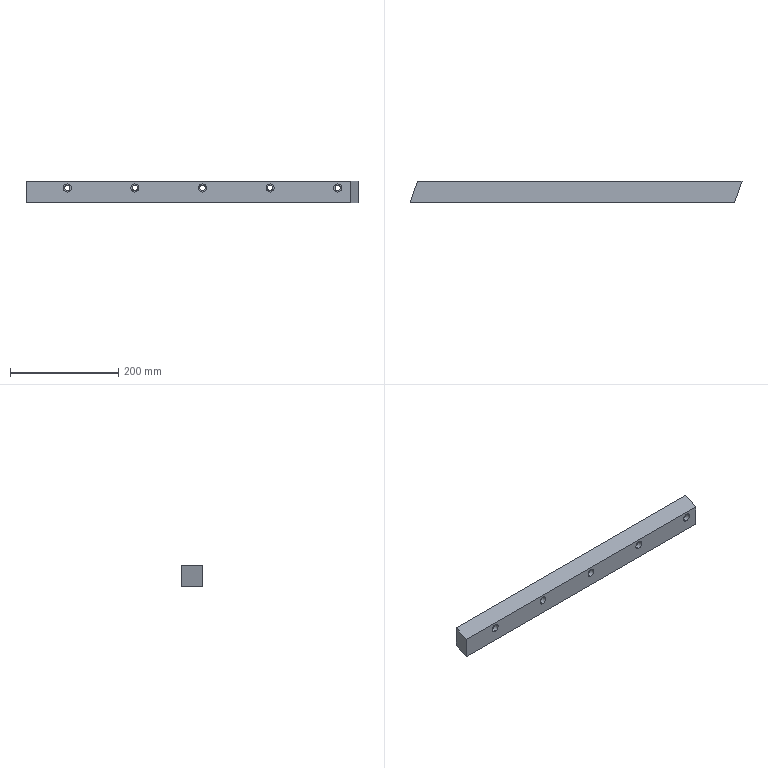Part | STEP file | MHH043906 | 1 solid | 31 faces | box 613.8 x 39 x 39 mm | volume 892867 mm3 | cylinder 20 | plane 11 | commonest cylinder face diameters 10 x10 15 x10
STEP:
#1=CARTESIAN_POINT('',(187.5,-30.,34.5));
#2=VERTEX_POINT('',#1);
#3=CARTESIAN_POINT('',(187.5,-30.,19.5));
#4=VERTEX_POINT('',#3);
#5=CARTESIAN_POINT('',(187.5,-30.,27.));
#6=DIRECTION('',(0.,-1.,0.));
#7=DIRECTION('',(0.,0.,-1.));
#8=AXIS2_PLACEMENT_3D('',#5,#6,#7);
#9=CIRCLE('',#8,7.5);
#10=EDGE_CURVE('',#2,#4,#9,.T.);
#11=ORIENTED_EDGE('',*,*,#10,.F.);
#12=CARTESIAN_POINT('',(187.5,-39.,34.5));
#13=VERTEX_POINT('',#12);
#14=CARTESIAN_POINT('',(187.5,-39.,34.5));
#15=DIRECTION('',(0.,-1.,0.));
#16=VECTOR('',#15,1000.);
#17=LINE('',#14,#16);
#18=EDGE_CURVE('',#2,#13,#17,.T.);
#19=ORIENTED_EDGE('',*,*,#18,.T.);
#20=CARTESIAN_POINT('',(187.5,-39.,19.5));
#21=VERTEX_POINT('',#20);
#22=CARTESIAN_POINT('',(187.5,-39.,27.));
#23=DIRECTION('',(0.,-1.,0.));
#24=DIRECTION('',(0.,0.,-1.));
#25=AXIS2_PLACEMENT_3D('',#22,#23,#24);
#26=CIRCLE('',#25,7.5);
#27=EDGE_CURVE('',#13,#21,#26,.T.);
#28=ORIENTED_EDGE('',*,*,#27,.T.);
#29=CARTESIAN_POINT('',(187.5,-39.,19.5));
#30=DIRECTION('',(0.,-1.,0.));
#31=VECTOR('',#30,1000.);
#32=LINE('',#29,#31);
#33=EDGE_CURVE('',#4,#21,#32,.T.);
#34=ORIENTED_EDGE('',*,*,#33,.F.);
#35=EDGE_LOOP('',(#11,#19,#28,#34));
#36=FACE_OUTER_BOUND('',#35,.T.);
#37=CARTESIAN_POINT('',(187.5,-39.,27.));
#38=DIRECTION('',(0.,-1.,0.));
#39=DIRECTION('',(0.,0.,-1.));
#40=AXIS2_PLACEMENT_3D('',#37,#38,#39);
#41=CYLINDRICAL_SURFACE('',#40,7.5);
#42=ADVANCED_FACE('',(#36),#41,.F.);
#43=CARTESIAN_POINT('',(187.5,0.,32.));
#44=VERTEX_POINT('',#43);
#45=CARTESIAN_POINT('',(187.5,0.,22.));
#46=VERTEX_POINT('',#45);
#47=CARTESIAN_POINT('',(187.5,0.,27.));
#48=DIRECTION('',(0.,-1.,0.));
#49=DIRECTION('',(0.,0.,-1.));
#50=AXIS2_PLACEMENT_3D('',#47,#48,#49);
#51=CIRCLE('',#50,5.);
#52=EDGE_CURVE('',#44,#46,#51,.T.);
#53=ORIENTED_EDGE('',*,*,#52,.F.);
#54=CARTESIAN_POINT('',(187.5,-30.,32.));
#55=VERTEX_POINT('',#54);
#56=CARTESIAN_POINT('',(187.5,-39.,32.));
#57=DIRECTION('',(0.,-1.,0.));
#58=VECTOR('',#57,1000.);
#59=LINE('',#56,#58);
#60=EDGE_CURVE('',#44,#55,#59,.T.);
#61=ORIENTED_EDGE('',*,*,#60,.T.);
#62=CARTESIAN_POINT('',(187.5,-30.,22.));
#63=VERTEX_POINT('',#62);
#64=CARTESIAN_POINT('',(187.5,-30.,27.));
#65=DIRECTION('',(0.,-1.,0.));
#66=DIRECTION('',(0.,0.,-1.));
#67=AXIS2_PLACEMENT_3D('',#64,#65,#66);
#68=CIRCLE('',#67,5.);
#69=EDGE_CURVE('',#55,#63,#68,.T.);
#70=ORIENTED_EDGE('',*,*,#69,.T.);
#71=CARTESIAN_POINT('',(187.5,-39.,22.));
#72=DIRECTION('',(0.,-1.,0.));
#73=VECTOR('',#72,1000.);
#74=LINE('',#71,#73);
#75=EDGE_CURVE('',#46,#63,#74,.T.);
#76=ORIENTED_EDGE('',*,*,#75,.F.);
#77=EDGE_LOOP('',(#53,#61,#70,#76));
#78=FACE_OUTER_BOUND('',#77,.T.);
#79=CARTESIAN_POINT('',(187.5,-39.,27.));
#80=DIRECTION('',(0.,-1.,0.));
#81=DIRECTION('',(0.,0.,-1.));
#82=AXIS2_PLACEMENT_3D('',#79,#80,#81);
#83=CYLINDRICAL_SURFACE('',#82,5.);
#84=ADVANCED_FACE('',(#78),#83,.F.);
#85=CARTESIAN_POINT('',(62.5,-30.,34.5));
#86=VERTEX_POINT('',#85);
#87=CARTESIAN_POINT('',(62.5,-30.,19.5));
#88=VERTEX_POINT('',#87);
#89=CARTESIAN_POINT('',(62.5,-30.,27.));
#90=DIRECTION('',(0.,-1.,0.));
#91=DIRECTION('',(0.,0.,-1.));
#92=AXIS2_PLACEMENT_3D('',#89,#90,#91);
#93=CIRCLE('',#92,7.5);
#94=EDGE_CURVE('',#86,#88,#93,.T.);
#95=ORIENTED_EDGE('',*,*,#94,.F.);
#96=CARTESIAN_POINT('',(62.5,-39.,34.5));
#97=VERTEX_POINT('',#96);
#98=CARTESIAN_POINT('',(62.5,-39.,34.5));
#99=DIRECTION('',(0.,-1.,0.));
#100=VECTOR('',#99,1000.);
#101=LINE('',#98,#100);
#102=EDGE_CURVE('',#86,#97,#101,.T.);
#103=ORIENTED_EDGE('',*,*,#102,.T.);
#104=CARTESIAN_POINT('',(62.5,-39.,19.5));
#105=VERTEX_POINT('',#104);
#106=CARTESIAN_POINT('',(62.5,-39.,27.));
#107=DIRECTION('',(0.,-1.,0.));
#108=DIRECTION('',(0.,0.,-1.));
#109=AXIS2_PLACEMENT_3D('',#106,#107,#108);
#110=CIRCLE('',#109,7.5);
#111=EDGE_CURVE('',#97,#105,#110,.T.);
#112=ORIENTED_EDGE('',*,*,#111,.T.);
#113=CARTESIAN_POINT('',(62.5,-39.,19.5));
#114=DIRECTION('',(0.,-1.,0.));
#115=VECTOR('',#114,1000.);
#116=LINE('',#113,#115);
#117=EDGE_CURVE('',#88,#105,#116,.T.);
#118=ORIENTED_EDGE('',*,*,#117,.F.);
#119=EDGE_LOOP('',(#95,#103,#112,#118));
#120=FACE_OUTER_BOUND('',#119,.T.);
#121=CARTESIAN_POINT('',(62.5,-39.,27.));
#122=DIRECTION('',(0.,-1.,0.));
#123=DIRECTION('',(0.,0.,-1.));
#124=AXIS2_PLACEMENT_3D('',#121,#122,#123);
#125=CYLINDRICAL_SURFACE('',#124,7.5);
#126=ADVANCED_FACE('',(#120),#125,.F.);
#127=CARTESIAN_POINT('',(62.5,0.,32.));
#128=VERTEX_POINT('',#127);
#129=CARTESIAN_POINT('',(62.5,0.,22.));
#130=VERTEX_POINT('',#129);
#131=CARTESIAN_POINT('',(62.5,0.,27.));
#132=DIRECTION('',(0.,-1.,0.));
#133=DIRECTION('',(0.,0.,-1.));
#134=AXIS2_PLACEMENT_3D('',#131,#132,#133);
#135=CIRCLE('',#134,5.);
#136=EDGE_CURVE('',#128,#130,#135,.T.);
#137=ORIENTED_EDGE('',*,*,#136,.F.);
#138=CARTESIAN_POINT('',(62.5,-30.,32.));
#139=VERTEX_POINT('',#138);
#140=CARTESIAN_POINT('',(62.5,-39.,32.));
#141=DIRECTION('',(0.,-1.,0.));
#142=VECTOR('',#141,1000.);
#143=LINE('',#140,#142);
#144=EDGE_CURVE('',#128,#139,#143,.T.);
#145=ORIENTED_EDGE('',*,*,#144,.T.);
#146=CARTESIAN_POINT('',(62.5,-30.,22.));
#147=VERTEX_POINT('',#146);
#148=CARTESIAN_POINT('',(62.5,-30.,27.));
#149=DIRECTION('',(0.,-1.,0.));
#150=DIRECTION('',(0.,0.,-1.));
#151=AXIS2_PLACEMENT_3D('',#148,#149,#150);
#152=CIRCLE('',#151,5.);
#153=EDGE_CURVE('',#139,#147,#152,.T.);
#154=ORIENTED_EDGE('',*,*,#153,.T.);
#155=CARTESIAN_POINT('',(62.5,-39.,22.));
#156=DIRECTION('',(0.,-1.,0.));
#157=VECTOR('',#156,1000.);
#158=LINE('',#155,#157);
#159=EDGE_CURVE('',#130,#147,#158,.T.);
#160=ORIENTED_EDGE('',*,*,#159,.F.);
#161=EDGE_LOOP('',(#137,#145,#154,#160));
#162=FACE_OUTER_BOUND('',#161,.T.);
#163=CARTESIAN_POINT('',(62.5,-39.,27.));
#164=DIRECTION('',(0.,-1.,0.));
#165=DIRECTION('',(0.,0.,-1.));
#166=AXIS2_PLACEMENT_3D('',#163,#164,#165);
#167=CYLINDRICAL_SURFACE('',#166,5.);
#168=ADVANCED_FACE('',(#162),#167,.F.);
#169=CARTESIAN_POINT('',(312.5,0.,32.));
#170=VERTEX_POINT('',#169);
#171=CARTESIAN_POINT('',(312.5,0.,22.));
#172=VERTEX_POINT('',#171);
#173=CARTESIAN_POINT('',(312.5,0.,27.));
#174=DIRECTION('',(0.,-1.,0.));
#175=DIRECTION('',(0.,0.,-1.));
#176=AXIS2_PLACEMENT_3D('',#173,#174,#175);
#177=CIRCLE('',#176,5.);
#178=EDGE_CURVE('',#170,#172,#177,.T.);
#179=ORIENTED_EDGE('',*,*,#178,.F.);
#180=CARTESIAN_POINT('',(312.5,-30.,32.));
#181=VERTEX_POINT('',#180);
#182=CARTESIAN_POINT('',(312.5,-39.,32.));
#183=DIRECTION('',(0.,-1.,0.));
#184=VECTOR('',#183,1000.);
#185=LINE('',#182,#184);
#186=EDGE_CURVE('',#170,#181,#185,.T.);
#187=ORIENTED_EDGE('',*,*,#186,.T.);
#188=CARTESIAN_POINT('',(312.5,-30.,22.));
#189=VERTEX_POINT('',#188);
#190=CARTESIAN_POINT('',(312.5,-30.,27.));
#191=DIRECTION('',(0.,-1.,0.));
#192=DIRECTION('',(0.,0.,-1.));
#193=AXIS2_PLACEMENT_3D('',#190,#191,#192);
#194=CIRCLE('',#193,5.);
#195=EDGE_CURVE('',#181,#189,#194,.T.);
#196=ORIENTED_EDGE('',*,*,#195,.T.);
#197=CARTESIAN_POINT('',(312.5,-39.,22.));
#198=DIRECTION('',(0.,-1.,0.));
#199=VECTOR('',#198,1000.);
#200=LINE('',#197,#199);
#201=EDGE_CURVE('',#172,#189,#200,.T.);
#202=ORIENTED_EDGE('',*,*,#201,.F.);
#203=EDGE_LOOP('',(#179,#187,#196,#202));
#204=FACE_OUTER_BOUND('',#203,.T.);
#205=CARTESIAN_POINT('',(312.5,-39.,27.));
#206=DIRECTION('',(0.,-1.,0.));
#207=DIRECTION('',(0.,0.,-1.));
#208=AXIS2_PLACEMENT_3D('',#205,#206,#207);
#209=CYLINDRICAL_SURFACE('',#208,5.);
#210=ADVANCED_FACE('',(#204),#209,.F.);
#211=CARTESIAN_POINT('',(312.5,-30.,34.5));
#212=VERTEX_POINT('',#211);
#213=CARTESIAN_POINT('',(312.5,-30.,19.5));
#214=VERTEX_POINT('',#213);
#215=CARTESIAN_POINT('',(312.5,-30.,27.));
#216=DIRECTION('',(0.,-1.,0.));
#217=DIRECTION('',(0.,0.,-1.));
#218=AXIS2_PLACEMENT_3D('',#215,#216,#217);
#219=CIRCLE('',#218,7.5);
#220=EDGE_CURVE('',#212,#214,#219,.T.);
#221=ORIENTED_EDGE('',*,*,#220,.F.);
#222=CARTESIAN_POINT('',(312.5,-39.,34.5));
#223=VERTEX_POINT('',#222);
#224=CARTESIAN_POINT('',(312.5,-39.,34.5));
#225=DIRECTION('',(0.,-1.,0.));
#226=VECTOR('',#225,1000.);
#227=LINE('',#224,#226);
#228=EDGE_CURVE('',#212,#223,#227,.T.);
#229=ORIENTED_EDGE('',*,*,#228,.T.);
#230=CARTESIAN_POINT('',(312.5,-39.,19.5));
#231=VERTEX_POINT('',#230);
#232=CARTESIAN_POINT('',(312.5,-39.,27.));
#233=DIRECTION('',(0.,-1.,0.));
#234=DIRECTION('',(0.,0.,-1.));
#235=AXIS2_PLACEMENT_3D('',#232,#233,#234);
#236=CIRCLE('',#235,7.5);
#237=EDGE_CURVE('',#223,#231,#236,.T.);
#238=ORIENTED_EDGE('',*,*,#237,.T.);
#239=CARTESIAN_POINT('',(312.5,-39.,19.5));
#240=DIRECTION('',(0.,-1.,0.));
#241=VECTOR('',#240,1000.);
#242=LINE('',#239,#241);
#243=EDGE_CURVE('',#214,#231,#242,.T.);
#244=ORIENTED_EDGE('',*,*,#243,.F.);
#245=EDGE_LOOP('',(#221,#229,#238,#244));
#246=FACE_OUTER_BOUND('',#245,.T.);
#247=CARTESIAN_POINT('',(312.5,-39.,27.));
#248=DIRECTION('',(0.,-1.,0.));
#249=DIRECTION('',(0.,0.,-1.));
#250=AXIS2_PLACEMENT_3D('',#247,#248,#249);
#251=CYLINDRICAL_SURFACE('',#250,7.5);
#252=ADVANCED_FACE('',(#246),#251,.F.);
#253=CARTESIAN_POINT('',(437.5,0.,32.));
#254=VERTEX_POINT('',#253);
#255=CARTESIAN_POINT('',(437.5,0.,22.));
#256=VERTEX_POINT('',#255);
#257=CARTESIAN_POINT('',(437.5,0.,27.));
#258=DIRECTION('',(0.,-1.,0.));
#259=DIRECTION('',(0.,0.,-1.));
#260=AXIS2_PLACEMENT_3D('',#257,#258,#259);
#261=CIRCLE('',#260,5.);
#262=EDGE_CURVE('',#254,#256,#261,.T.);
#263=ORIENTED_EDGE('',*,*,#262,.F.);
#264=CARTESIAN_POINT('',(437.5,-30.,32.));
#265=VERTEX_POINT('',#264);
#266=CARTESIAN_POINT('',(437.5,-39.,32.));
#267=DIRECTION('',(0.,-1.,0.));
#268=VECTOR('',#267,1000.);
#269=LINE('',#266,#268);
#270=EDGE_CURVE('',#254,#265,#269,.T.);
#271=ORIENTED_EDGE('',*,*,#270,.T.);
#272=CARTESIAN_POINT('',(437.5,-30.,22.));
#273=VERTEX_POINT('',#272);
#274=CARTESIAN_POINT('',(437.5,-30.,27.));
#275=DIRECTION('',(0.,-1.,0.));
#276=DIRECTION('',(0.,0.,-1.));
#277=AXIS2_PLACEMENT_3D('',#274,#275,#276);
#278=CIRCLE('',#277,5.);
#279=EDGE_CURVE('',#265,#273,#278,.T.);
#280=ORIENTED_EDGE('',*,*,#279,.T.);
#281=CARTESIAN_POINT('',(437.5,-39.,22.));
#282=DIRECTION('',(0.,-1.,0.));
#283=VECTOR('',#282,1000.);
#284=LINE('',#281,#283);
#285=EDGE_CURVE('',#256,#273,#284,.T.);
#286=ORIENTED_EDGE('',*,*,#285,.F.);
#287=EDGE_LOOP('',(#263,#271,#280,#286));
#288=FACE_OUTER_BOUND('',#287,.T.);
#289=CARTESIAN_POINT('',(437.5,-39.,27.));
#290=DIRECTION('',(0.,-1.,0.));
#291=DIRECTION('',(0.,0.,-1.));
#292=AXIS2_PLACEMENT_3D('',#289,#290,#291);
#293=CYLINDRICAL_SURFACE('',#292,5.);
#294=ADVANCED_FACE('',(#288),#293,.F.);
#295=CARTESIAN_POINT('',(437.5,-30.,34.5));
#296=VERTEX_POINT('',#295);
#297=CARTESIAN_POINT('',(437.5,-30.,19.5));
#298=VERTEX_POINT('',#297);
#299=CARTESIAN_POINT('',(437.5,-30.,27.));
#300=DIRECTION('',(0.,-1.,0.));
#301=DIRECTION('',(0.,0.,-1.));
#302=AXIS2_PLACEMENT_3D('',#299,#300,#301);
#303=CIRCLE('',#302,7.5);
#304=EDGE_CURVE('',#296,#298,#303,.T.);
#305=ORIENTED_EDGE('',*,*,#304,.F.);
#306=CARTESIAN_POINT('',(437.5,-39.,34.5));
#307=VERTEX_POINT('',#306);
#308=CARTESIAN_POINT('',(437.5,-39.,34.5));
#309=DIRECTION('',(0.,-1.,0.));
#310=VECTOR('',#309,1000.);
#311=LINE('',#308,#310);
#312=EDGE_CURVE('',#296,#307,#311,.T.);
#313=ORIENTED_EDGE('',*,*,#312,.T.);
#314=CARTESIAN_POINT('',(437.5,-39.,19.5));
#315=VERTEX_POINT('',#314);
#316=CARTESIAN_POINT('',(437.5,-39.,27.));
#317=DIRECTION('',(0.,-1.,0.));
#318=DIRECTION('',(0.,0.,-1.));
#319=AXIS2_PLACEMENT_3D('',#316,#317,#318);
#320=CIRCLE('',#319,7.5);
#321=EDGE_CURVE('',#307,#315,#320,.T.);
#322=ORIENTED_EDGE('',*,*,#321,.T.);
#323=CARTESIAN_POINT('',(437.5,-39.,19.5));
#324=DIRECTION('',(0.,-1.,0.));
#325=VECTOR('',#324,1000.);
#326=LINE('',#323,#325);
#327=EDGE_CURVE('',#298,#315,#326,.T.);
#328=ORIENTED_EDGE('',*,*,#327,.F.);
#329=EDGE_LOOP('',(#305,#313,#322,#328));
#330=FACE_OUTER_BOUND('',#329,.T.);
#331=CARTESIAN_POINT('',(437.5,-39.,27.));
#332=DIRECTION('',(0.,-1.,0.));
#333=DIRECTION('',(0.,0.,-1.));
#334=AXIS2_PLACEMENT_3D('',#331,#332,#333);
#335=CYLINDRICAL_SURFACE('',#334,7.5);
#336=ADVANCED_FACE('',(#330),#335,.F.);
#337=CARTESIAN_POINT('',(562.5,0.,32.));
#338=VERTEX_POINT('',#337);
#339=CARTESIAN_POINT('',(562.5,0.,22.));
#340=VERTEX_POINT('',#339);
#341=CARTESIAN_POINT('',(562.5,0.,27.));
#342=DIRECTION('',(0.,-1.,0.));
#343=DIRECTION('',(0.,0.,-1.));
#344=AXIS2_PLACEMENT_3D('',#341,#342,#343);
#345=CIRCLE('',#344,5.);
#346=EDGE_CURVE('',#338,#340,#345,.T.);
#347=ORIENTED_EDGE('',*,*,#346,.F.);
#348=CARTESIAN_POINT('',(562.5,-30.,32.));
#349=VERTEX_POINT('',#348);
#350=CARTESIAN_POINT('',(562.5,-39.,32.));
#351=DIRECTION('',(0.,-1.,0.));
#352=VECTOR('',#351,1000.);
#353=LINE('',#350,#352);
#354=EDGE_CURVE('',#338,#349,#353,.T.);
#355=ORIENTED_EDGE('',*,*,#354,.T.);
#356=CARTESIAN_POINT('',(562.5,-30.,22.));
#357=VERTEX_POINT('',#356);
#358=CARTESIAN_POINT('',(562.5,-30.,27.));
#359=DIRECTION('',(0.,-1.,0.));
#360=DIRECTION('',(0.,0.,-1.));
#361=AXIS2_PLACEMENT_3D('',#358,#359,#360);
#362=CIRCLE('',#361,5.);
#363=EDGE_CURVE('',#349,#357,#362,.T.);
#364=ORIENTED_EDGE('',*,*,#363,.T.);
#365=CARTESIAN_POINT('',(562.5,-39.,22.));
#366=DIRECTION('',(0.,-1.,0.));
#367=VECTOR('',#366,1000.);
#368=LINE('',#365,#367);
#369=EDGE_CURVE('',#340,#357,#368,.T.);
#370=ORIENTED_EDGE('',*,*,#369,.F.);
#371=EDGE_LOOP('',(#347,#355,#364,#370));
#372=FACE_OUTER_BOUND('',#371,.T.);
#373=CARTESIAN_POINT('',(562.5,-39.,27.));
#374=DIRECTION('',(0.,-1.,0.));
#375=DIRECTION('',(0.,0.,-1.));
#376=AXIS2_PLACEMENT_3D('',#373,#374,#375);
#377=CYLINDRICAL_SURFACE('',#376,5.);
#378=ADVANCED_FACE('',(#372),#377,.F.);
#379=CARTESIAN_POINT('',(562.5,-30.,34.5));
#380=VERTEX_POINT('',#379);
#381=CARTESIAN_POINT('',(562.5,-30.,19.5));
#382=VERTEX_POINT('',#381);
#383=CARTESIAN_POINT('',(562.5,-30.,27.));
#384=DIRECTION('',(0.,-1.,0.));
#385=DIRECTION('',(0.,0.,-1.));
#386=AXIS2_PLACEMENT_3D('',#383,#384,#385);
#387=CIRCLE('',#386,7.5);
#388=EDGE_CURVE('',#380,#382,#387,.T.);
#389=ORIENTED_EDGE('',*,*,#388,.F.);
#390=CARTESIAN_POINT('',(562.5,-39.,34.5));
#391=VERTEX_POINT('',#390);
#392=CARTESIAN_POINT('',(562.5,-39.,34.5));
#393=DIRECTION('',(0.,-1.,0.));
#394=VECTOR('',#393,1000.);
#395=LINE('',#392,#394);
#396=EDGE_CURVE('',#380,#391,#395,.T.);
#397=ORIENTED_EDGE('',*,*,#396,.T.);
#398=CARTESIAN_POINT('',(562.5,-39.,19.5));
#399=VERTEX_POINT('',#398);
#400=CARTESIAN_POINT('',(562.5,-39.,27.));
#401=DIRECTION('',(0.,-1.,0.));
#402=DIRECTION('',(0.,0.,-1.));
#403=AXIS2_PLACEMENT_3D('',#400,#401,#402);
#404=CIRCLE('',#403,7.5);
#405=EDGE_CURVE('',#391,#399,#404,.T.);
#406=ORIENTED_EDGE('',*,*,#405,.T.);
#407=CARTESIAN_POINT('',(562.5,-39.,19.5));
#408=DIRECTION('',(0.,-1.,0.));
#409=VECTOR('',#408,1000.);
#410=LINE('',#407,#409);
#411=EDGE_CURVE('',#382,#399,#410,.T.);
#412=ORIENTED_EDGE('',*,*,#411,.F.);
#413=EDGE_LOOP('',(#389,#397,#406,#412));
#414=FACE_OUTER_BOUND('',#413,.T.);
#415=CARTESIAN_POINT('',(562.5,-39.,27.));
#416=DIRECTION('',(0.,-1.,0.));
#417=DIRECTION('',(0.,0.,-1.));
#418=AXIS2_PLACEMENT_3D('',#415,#416,#417);
#419=CYLINDRICAL_SURFACE('',#418,7.5);
#420=ADVANCED_FACE('',(#414),#419,.F.);
#421=ORIENTED_EDGE('',*,*,#396,.F.);
#422=CARTESIAN_POINT('',(562.5,-30.,27.));
#423=DIRECTION('',(0.,-1.,0.));
#424=DIRECTION('',(0.,0.,-1.));
#425=AXIS2_PLACEMENT_3D('',#422,#423,#424);
#426=CIRCLE('',#425,7.5);
#427=EDGE_CURVE('',#382,#380,#426,.T.);
#428=ORIENTED_EDGE('',*,*,#427,.F.);
#429=ORIENTED_EDGE('',*,*,#411,.T.);
#430=CARTESIAN_POINT('',(562.5,-39.,27.));
#431=DIRECTION('',(0.,-1.,0.));
#432=DIRECTION('',(0.,0.,-1.));
#433=AXIS2_PLACEMENT_3D('',#430,#431,#432);
#434=CIRCLE('',#433,7.5);
#435=EDGE_CURVE('',#399,#391,#434,.T.);
#436=ORIENTED_EDGE('',*,*,#435,.T.);
#437=EDGE_LOOP('',(#421,#428,#429,#436));
#438=FACE_OUTER_BOUND('',#437,.T.);
#439=CARTESIAN_POINT('',(562.5,-39.,27.));
#440=DIRECTION('',(0.,-1.,0.));
#441=DIRECTION('',(0.,0.,-1.));
#442=AXIS2_PLACEMENT_3D('',#439,#440,#441);
#443=CYLINDRICAL_SURFACE('',#442,7.5);
#444=ADVANCED_FACE('',(#438),#443,.F.);
#445=CARTESIAN_POINT('',(562.5,-30.,27.));
#446=DIRECTION('',(0.,-1.,0.));
#447=DIRECTION('',(0.,0.,-1.));
#448=AXIS2_PLACEMENT_3D('',#445,#446,#447);
#449=CIRCLE('',#448,5.);
#450=EDGE_CURVE('',#357,#349,#449,.T.);
#451=ORIENTED_EDGE('',*,*,#450,.F.);
#452=ORIENTED_EDGE('',*,*,#363,.F.);
#453=EDGE_LOOP('',(#451,#452));
#454=FACE_BOUND('',#453,.T.);
#455=ORIENTED_EDGE('',*,*,#427,.T.);
#456=ORIENTED_EDGE('',*,*,#388,.T.);
#457=EDGE_LOOP('',(#455,#456));
#458=FACE_OUTER_BOUND('',#457,.T.);
#459=CARTESIAN_POINT('',(567.5,-30.,27.));
#460=DIRECTION('',(0.,1.,0.));
#461=DIRECTION('',(0.,0.,1.));
#462=AXIS2_PLACEMENT_3D('',#459,#460,#461);
#463=PLANE('',#462);
#464=ADVANCED_FACE('',(#454,#458),#463,.F.);
#465=ORIENTED_EDGE('',*,*,#354,.F.);
#466=CARTESIAN_POINT('',(562.5,0.,27.));
#467=DIRECTION('',(0.,-1.,0.));
#468=DIRECTION('',(0.,0.,-1.));
#469=AXIS2_PLACEMENT_3D('',#466,#467,#468);
#470=CIRCLE('',#469,5.);
#471=EDGE_CURVE('',#340,#338,#470,.T.);
#472=ORIENTED_EDGE('',*,*,#471,.F.);
#473=ORIENTED_EDGE('',*,*,#369,.T.);
#474=ORIENTED_EDGE('',*,*,#450,.T.);
#475=EDGE_LOOP('',(#465,#472,#473,#474));
#476=FACE_OUTER_BOUND('',#475,.T.);
#477=CARTESIAN_POINT('',(562.5,-39.,27.));
#478=DIRECTION('',(0.,-1.,0.));
#479=DIRECTION('',(0.,0.,-1.));
#480=AXIS2_PLACEMENT_3D('',#477,#478,#479);
#481=CYLINDRICAL_SURFACE('',#480,5.);
#482=ADVANCED_FACE('',(#476),#481,.F.);
#483=ORIENTED_EDGE('',*,*,#312,.F.);
#484=CARTESIAN_POINT('',(437.5,-30.,27.));
#485=DIRECTION('',(0.,-1.,0.));
#486=DIRECTION('',(0.,0.,-1.));
#487=AXIS2_PLACEMENT_3D('',#484,#485,#486);
#488=CIRCLE('',#487,7.5);
#489=EDGE_CURVE('',#298,#296,#488,.T.);
#490=ORIENTED_EDGE('',*,*,#489,.F.);
#491=ORIENTED_EDGE('',*,*,#327,.T.);
#492=CARTESIAN_POINT('',(437.5,-39.,27.));
#493=DIRECTION('',(0.,-1.,0.));
#494=DIRECTION('',(0.,0.,-1.));
#495=AXIS2_PLACEMENT_3D('',#492,#493,#494);
#496=CIRCLE('',#495,7.5);
#497=EDGE_CURVE('',#315,#307,#496,.T.);
#498=ORIENTED_EDGE('',*,*,#497,.T.);
#499=EDGE_LOOP('',(#483,#490,#491,#498));
#500=FACE_OUTER_BOUND('',#499,.T.);
#501=CARTESIAN_POINT('',(437.5,-39.,27.));
#502=DIRECTION('',(0.,-1.,0.));
#503=DIRECTION('',(0.,0.,-1.));
#504=AXIS2_PLACEMENT_3D('',#501,#502,#503);
#505=CYLINDRICAL_SURFACE('',#504,7.5);
#506=ADVANCED_FACE('',(#500),#505,.F.);
#507=CARTESIAN_POINT('',(437.5,-30.,27.));
#508=DIRECTION('',(0.,-1.,0.));
#509=DIRECTION('',(0.,0.,-1.));
#510=AXIS2_PLACEMENT_3D('',#507,#508,#509);
#511=CIRCLE('',#510,5.);
#512=EDGE_CURVE('',#273,#265,#511,.T.);
#513=ORIENTED_EDGE('',*,*,#512,.F.);
#514=ORIENTED_EDGE('',*,*,#279,.F.);
#515=EDGE_LOOP('',(#513,#514));
#516=FACE_BOUND('',#515,.T.);
#517=ORIENTED_EDGE('',*,*,#489,.T.);
#518=ORIENTED_EDGE('',*,*,#304,.T.);
#519=EDGE_LOOP('',(#517,#518));
#520=FACE_OUTER_BOUND('',#519,.T.);
#521=CARTESIAN_POINT('',(442.5,-30.,27.));
#522=DIRECTION('',(0.,1.,0.));
#523=DIRECTION('',(0.,0.,1.));
#524=AXIS2_PLACEMENT_3D('',#521,#522,#523);
#525=PLANE('',#524);
#526=ADVANCED_FACE('',(#516,#520),#525,.F.);
#527=ORIENTED_EDGE('',*,*,#270,.F.);
#528=CARTESIAN_POINT('',(437.5,0.,27.));
#529=DIRECTION('',(0.,-1.,0.));
#530=DIRECTION('',(0.,0.,-1.));
#531=AXIS2_PLACEMENT_3D('',#528,#529,#530);
#532=CIRCLE('',#531,5.);
#533=EDGE_CURVE('',#256,#254,#532,.T.);
#534=ORIENTED_EDGE('',*,*,#533,.F.);
#535=ORIENTED_EDGE('',*,*,#285,.T.);
#536=ORIENTED_EDGE('',*,*,#512,.T.);
#537=EDGE_LOOP('',(#527,#534,#535,#536));
#538=FACE_OUTER_BOUND('',#537,.T.);
#539=CARTESIAN_POINT('',(437.5,-39.,27.));
#540=DIRECTION('',(0.,-1.,0.));
#541=DIRECTION('',(0.,0.,-1.));
#542=AXIS2_PLACEMENT_3D('',#539,#540,#541);
#543=CYLINDRICAL_SURFACE('',#542,5.);
#544=ADVANCED_FACE('',(#538),#543,.F.);
#545=ORIENTED_EDGE('',*,*,#228,.F.);
#546=CARTESIAN_POINT('',(312.5,-30.,27.));
#547=DIRECTION('',(0.,-1.,0.));
#548=DIRECTION('',(0.,0.,-1.));
#549=AXIS2_PLACEMENT_3D('',#546,#547,#548);
#550=CIRCLE('',#549,7.5);
#551=EDGE_CURVE('',#214,#212,#550,.T.);
#552=ORIENTED_EDGE('',*,*,#551,.F.);
#553=ORIENTED_EDGE('',*,*,#243,.T.);
#554=CARTESIAN_POINT('',(312.5,-39.,27.));
#555=DIRECTION('',(0.,-1.,0.));
#556=DIRECTION('',(0.,0.,-1.));
#557=AXIS2_PLACEMENT_3D('',#554,#555,#556);
#558=CIRCLE('',#557,7.5);
#559=EDGE_CURVE('',#231,#223,#558,.T.);
#560=ORIENTED_EDGE('',*,*,#559,.T.);
#561=EDGE_LOOP('',(#545,#552,#553,#560));
#562=FACE_OUTER_BOUND('',#561,.T.);
#563=CARTESIAN_POINT('',(312.5,-39.,27.));
#564=DIRECTION('',(0.,-1.,0.));
#565=DIRECTION('',(0.,0.,-1.));
#566=AXIS2_PLACEMENT_3D('',#563,#564,#565);
#567=CYLINDRICAL_SURFACE('',#566,7.5);
#568=ADVANCED_FACE('',(#562),#567,.F.);
#569=CARTESIAN_POINT('',(312.5,-30.,27.));
#570=DIRECTION('',(0.,-1.,0.));
#571=DIRECTION('',(0.,0.,-1.));
#572=AXIS2_PLACEMENT_3D('',#569,#570,#571);
#573=CIRCLE('',#572,5.);
#574=EDGE_CURVE('',#189,#181,#573,.T.);
#575=ORIENTED_EDGE('',*,*,#574,.F.);
#576=ORIENTED_EDGE('',*,*,#195,.F.);
#577=EDGE_LOOP('',(#575,#576));
#578=FACE_BOUND('',#577,.T.);
#579=ORIENTED_EDGE('',*,*,#551,.T.);
#580=ORIENTED_EDGE('',*,*,#220,.T.);
#581=EDGE_LOOP('',(#579,#580));
#582=FACE_OUTER_BOUND('',#581,.T.);
#583=CARTESIAN_POINT('',(317.5,-30.,27.));
#584=DIRECTION('',(0.,1.,0.));
#585=DIRECTION('',(0.,0.,1.));
#586=AXIS2_PLACEMENT_3D('',#583,#584,#585);
#587=PLANE('',#586);
#588=ADVANCED_FACE('',(#578,#582),#587,.F.);
#589=ORIENTED_EDGE('',*,*,#186,.F.);
#590=CARTESIAN_POINT('',(312.5,0.,27.));
#591=DIRECTION('',(0.,-1.,0.));
#592=DIRECTION('',(0.,0.,-1.));
#593=AXIS2_PLACEMENT_3D('',#590,#591,#592);
#594=CIRCLE('',#593,5.);
#595=EDGE_CURVE('',#172,#170,#594,.T.);
#596=ORIENTED_EDGE('',*,*,#595,.F.);
#597=ORIENTED_EDGE('',*,*,#201,.T.);
#598=ORIENTED_EDGE('',*,*,#574,.T.);
#599=EDGE_LOOP('',(#589,#596,#597,#598));
#600=FACE_OUTER_BOUND('',#599,.T.);
#601=CARTESIAN_POINT('',(312.5,-39.,27.));
#602=DIRECTION('',(0.,-1.,0.));
#603=DIRECTION('',(0.,0.,-1.));
#604=AXIS2_PLACEMENT_3D('',#601,#602,#603);
#605=CYLINDRICAL_SURFACE('',#604,5.);
#606=ADVANCED_FACE('',(#600),#605,.F.);
#607=CARTESIAN_POINT('',(187.5,0.,27.));
#608=DIRECTION('',(0.,-1.,0.));
#609=DIRECTION('',(0.,0.,-1.));
#610=AXIS2_PLACEMENT_3D('',#607,#608,#609);
#611=CIRCLE('',#610,5.);
#612=EDGE_CURVE('',#46,#44,#611,.T.);
#613=ORIENTED_EDGE('',*,*,#612,.T.);
#614=ORIENTED_EDGE('',*,*,#52,.T.);
#615=EDGE_LOOP('',(#613,#614));
#616=FACE_BOUND('',#615,.T.);
#617=CARTESIAN_POINT('',(62.5,0.,27.));
#618=DIRECTION('',(0.,-1.,0.));
#619=DIRECTION('',(0.,0.,-1.));
#620=AXIS2_PLACEMENT_3D('',#617,#618,#619);
#621=CIRCLE('',#620,5.);
#622=EDGE_CURVE('',#130,#128,#621,.T.);
#623=ORIENTED_EDGE('',*,*,#622,.T.);
#624=ORIENTED_EDGE('',*,*,#136,.T.);
#625=EDGE_LOOP('',(#623,#624));
#626=FACE_BOUND('',#625,.T.);
#627=CARTESIAN_POINT('',(600.,0.,0.));
#628=VERTEX_POINT('',#627);
#629=CARTESIAN_POINT('',(0.,0.,0.));
#630=VERTEX_POINT('',#629);
#631=CARTESIAN_POINT('',(600.,0.,0.));
#632=DIRECTION('',(-1.,0.,0.));
#633=VECTOR('',#632,1000.);
#634=LINE('',#631,#633);
#635=EDGE_CURVE('',#628,#630,#634,.T.);
#636=ORIENTED_EDGE('',*,*,#635,.T.);
#637=CARTESIAN_POINT('',(0.,0.,39.));
#638=VERTEX_POINT('',#637);
#639=CARTESIAN_POINT('',(0.,0.,39.));
#640=DIRECTION('',(0.,0.,-1.));
#641=VECTOR('',#640,1000.);
#642=LINE('',#639,#641);
#643=EDGE_CURVE('',#638,#630,#642,.T.);
#644=ORIENTED_EDGE('',*,*,#643,.F.);
#645=CARTESIAN_POINT('',(600.,0.,39.));
#646=VERTEX_POINT('',#645);
#647=CARTESIAN_POINT('',(600.,0.,39.));
#648=DIRECTION('',(-1.,0.,0.));
#649=VECTOR('',#648,1000.);
#650=LINE('',#647,#649);
#651=EDGE_CURVE('',#646,#638,#650,.T.);
#652=ORIENTED_EDGE('',*,*,#651,.F.);
#653=CARTESIAN_POINT('',(600.,0.,39.));
#654=DIRECTION('',(0.,0.,-1.));
#655=VECTOR('',#654,1000.);
#656=LINE('',#653,#655);
#657=EDGE_CURVE('',#646,#628,#656,.T.);
#658=ORIENTED_EDGE('',*,*,#657,.T.);
#659=EDGE_LOOP('',(#636,#644,#652,#658));
#660=FACE_OUTER_BOUND('',#659,.T.);
#661=ORIENTED_EDGE('',*,*,#595,.T.);
#662=ORIENTED_EDGE('',*,*,#178,.T.);
#663=EDGE_LOOP('',(#661,#662));
#664=FACE_BOUND('',#663,.T.);
#665=ORIENTED_EDGE('',*,*,#533,.T.);
#666=ORIENTED_EDGE('',*,*,#262,.T.);
#667=EDGE_LOOP('',(#665,#666));
#668=FACE_BOUND('',#667,.T.);
#669=ORIENTED_EDGE('',*,*,#471,.T.);
#670=ORIENTED_EDGE('',*,*,#346,.T.);
#671=EDGE_LOOP('',(#669,#670));
#672=FACE_BOUND('',#671,.T.);
#673=CARTESIAN_POINT('',(600.,0.,39.));
#674=DIRECTION('',(0.,-1.,0.));
#675=DIRECTION('',(1.,0.,0.));
#676=AXIS2_PLACEMENT_3D('',#673,#674,#675);
#677=PLANE('',#676);
#678=ADVANCED_FACE('',(#616,#626,#660,#664,#668,#672),#677,.F.);
#679=CARTESIAN_POINT('',(-13.8,-39.,0.));
#680=VERTEX_POINT('',#679);
#681=CARTESIAN_POINT('',(0.,0.,0.));
#682=DIRECTION('',(-0.3336,-0.9427,0.));
#683=VECTOR('',#682,1000.);
#684=LINE('',#681,#683);
#685=EDGE_CURVE('',#630,#680,#684,.T.);
#686=ORIENTED_EDGE('',*,*,#685,.T.);
#687=CARTESIAN_POINT('',(-13.8,-39.,39.));
#688=VERTEX_POINT('',#687);
#689=CARTESIAN_POINT('',(-13.8,-39.,39.));
#690=DIRECTION('',(0.,0.,-1.));
#691=VECTOR('',#690,1000.);
#692=LINE('',#689,#691);
#693=EDGE_CURVE('',#688,#680,#692,.T.);
#694=ORIENTED_EDGE('',*,*,#693,.F.);
#695=CARTESIAN_POINT('',(0.,0.,39.));
#696=DIRECTION('',(-0.3336,-0.9427,0.));
#697=VECTOR('',#696,1000.);
#698=LINE('',#695,#697);
#699=EDGE_CURVE('',#638,#688,#698,.T.);
#700=ORIENTED_EDGE('',*,*,#699,.F.);
#701=ORIENTED_EDGE('',*,*,#643,.T.);
#702=EDGE_LOOP('',(#686,#694,#700,#701));
#703=FACE_OUTER_BOUND('',#702,.T.);
#704=CARTESIAN_POINT('',(0.,0.,39.));
#705=DIRECTION('',(0.9427,-0.3336,0.));
#706=DIRECTION('',(0.3336,0.9427,0.));
#707=AXIS2_PLACEMENT_3D('',#704,#705,#706);
#708=PLANE('',#707);
#709=ADVANCED_FACE('',(#703),#708,.F.);
#710=CARTESIAN_POINT('',(187.5,-39.,27.));
#711=DIRECTION('',(0.,-1.,0.));
#712=DIRECTION('',(0.,0.,-1.));
#713=AXIS2_PLACEMENT_3D('',#710,#711,#712);
#714=CIRCLE('',#713,7.5);
#715=EDGE_CURVE('',#21,#13,#714,.T.);
#716=ORIENTED_EDGE('',*,*,#715,.F.);
#717=ORIENTED_EDGE('',*,*,#27,.F.);
#718=EDGE_LOOP('',(#716,#717));
#719=FACE_BOUND('',#718,.T.);
#720=CARTESIAN_POINT('',(62.5,-39.,27.));
#721=DIRECTION('',(0.,-1.,0.));
#722=DIRECTION('',(0.,0.,-1.));
#723=AXIS2_PLACEMENT_3D('',#720,#721,#722);
#724=CIRCLE('',#723,7.5);
#725=EDGE_CURVE('',#105,#97,#724,.T.);
#726=ORIENTED_EDGE('',*,*,#725,.F.);
#727=ORIENTED_EDGE('',*,*,#111,.F.);
#728=EDGE_LOOP('',(#726,#727));
#729=FACE_BOUND('',#728,.T.);
#730=CARTESIAN_POINT('',(586.2,-39.,0.));
#731=VERTEX_POINT('',#730);
#732=CARTESIAN_POINT('',(-13.8,-39.,0.));
#733=DIRECTION('',(1.,0.,0.));
#734=VECTOR('',#733,1000.);
#735=LINE('',#732,#734);
#736=EDGE_CURVE('',#680,#731,#735,.T.);
#737=ORIENTED_EDGE('',*,*,#736,.T.);
#738=CARTESIAN_POINT('',(586.2,-39.,39.));
#739=VERTEX_POINT('',#738);
#740=CARTESIAN_POINT('',(586.2,-39.,39.));
#741=DIRECTION('',(0.,0.,-1.));
#742=VECTOR('',#741,1000.);
#743=LINE('',#740,#742);
#744=EDGE_CURVE('',#739,#731,#743,.T.);
#745=ORIENTED_EDGE('',*,*,#744,.F.);
#746=CARTESIAN_POINT('',(-13.8,-39.,39.));
#747=DIRECTION('',(1.,0.,0.));
#748=VECTOR('',#747,1000.);
#749=LINE('',#746,#748);
#750=EDGE_CURVE('',#688,#739,#749,.T.);
#751=ORIENTED_EDGE('',*,*,#750,.F.);
#752=ORIENTED_EDGE('',*,*,#693,.T.);
#753=EDGE_LOOP('',(#737,#745,#751,#752));
#754=FACE_OUTER_BOUND('',#753,.T.);
#755=ORIENTED_EDGE('',*,*,#559,.F.);
#756=ORIENTED_EDGE('',*,*,#237,.F.);
#757=EDGE_LOOP('',(#755,#756));
#758=FACE_BOUND('',#757,.T.);
#759=ORIENTED_EDGE('',*,*,#497,.F.);
#760=ORIENTED_EDGE('',*,*,#321,.F.);
#761=EDGE_LOOP('',(#759,#760));
#762=FACE_BOUND('',#761,.T.);
#763=ORIENTED_EDGE('',*,*,#435,.F.);
#764=ORIENTED_EDGE('',*,*,#405,.F.);
#765=EDGE_LOOP('',(#763,#764));
#766=FACE_BOUND('',#765,.T.);
#767=CARTESIAN_POINT('',(-13.8,-39.,39.));
#768=DIRECTION('',(0.,1.,0.));
#769=DIRECTION('',(-1.,0.,0.));
#770=AXIS2_PLACEMENT_3D('',#767,#768,#769);
#771=PLANE('',#770);
#772=ADVANCED_FACE('',(#719,#729,#754,#758,#762,#766),#771,.F.);
#773=CARTESIAN_POINT('',(586.2,-39.,0.));
#774=DIRECTION('',(0.3336,0.9427,0.));
#775=VECTOR('',#774,1000.);
#776=LINE('',#773,#775);
#777=EDGE_CURVE('',#731,#628,#776,.T.);
#778=ORIENTED_EDGE('',*,*,#777,.T.);
#779=ORIENTED_EDGE('',*,*,#657,.F.);
#780=CARTESIAN_POINT('',(586.2,-39.,39.));
#781=DIRECTION('',(0.3336,0.9427,0.));
#782=VECTOR('',#781,1000.);
#783=LINE('',#780,#782);
#784=EDGE_CURVE('',#739,#646,#783,.T.);
#785=ORIENTED_EDGE('',*,*,#784,.F.);
#786=ORIENTED_EDGE('',*,*,#744,.T.);
#787=EDGE_LOOP('',(#778,#779,#785,#786));
#788=FACE_OUTER_BOUND('',#787,.T.);
#789=CARTESIAN_POINT('',(586.2,-39.,39.));
#790=DIRECTION('',(-0.9427,0.3336,0.));
#791=DIRECTION('',(-0.3336,-0.9427,0.));
#792=AXIS2_PLACEMENT_3D('',#789,#790,#791);
#793=PLANE('',#792);
#794=ADVANCED_FACE('',(#788),#793,.F.);
#795=ORIENTED_EDGE('',*,*,#651,.T.);
#796=ORIENTED_EDGE('',*,*,#699,.T.);
#797=ORIENTED_EDGE('',*,*,#750,.T.);
#798=ORIENTED_EDGE('',*,*,#784,.T.);
#799=EDGE_LOOP('',(#795,#796,#797,#798));
#800=FACE_OUTER_BOUND('',#799,.T.);
#801=CARTESIAN_POINT('',(0.,0.,39.));
#802=DIRECTION('',(0.,0.,1.));
#803=DIRECTION('',(1.,0.,0.));
#804=AXIS2_PLACEMENT_3D('',#801,#802,#803);
#805=PLANE('',#804);
#806=ADVANCED_FACE('',(#800),#805,.T.);
#807=ORIENTED_EDGE('',*,*,#635,.F.);
#808=ORIENTED_EDGE('',*,*,#777,.F.);
#809=ORIENTED_EDGE('',*,*,#736,.F.);
#810=ORIENTED_EDGE('',*,*,#685,.F.);
#811=EDGE_LOOP('',(#807,#808,#809,#810));
#812=FACE_OUTER_BOUND('',#811,.T.);
#813=CARTESIAN_POINT('',(0.,0.,0.));
#814=DIRECTION('',(0.,0.,1.));
#815=DIRECTION('',(1.,0.,0.));
#816=AXIS2_PLACEMENT_3D('',#813,#814,#815);
#817=PLANE('',#816);
#818=ADVANCED_FACE('',(#812),#817,.F.);
#819=ORIENTED_EDGE('',*,*,#144,.F.);
#820=ORIENTED_EDGE('',*,*,#622,.F.);
#821=ORIENTED_EDGE('',*,*,#159,.T.);
#822=CARTESIAN_POINT('',(62.5,-30.,27.));
#823=DIRECTION('',(0.,-1.,0.));
#824=DIRECTION('',(0.,0.,-1.));
#825=AXIS2_PLACEMENT_3D('',#822,#823,#824);
#826=CIRCLE('',#825,5.);
#827=EDGE_CURVE('',#147,#139,#826,.T.);
#828=ORIENTED_EDGE('',*,*,#827,.T.);
#829=EDGE_LOOP('',(#819,#820,#821,#828));
#830=FACE_OUTER_BOUND('',#829,.T.);
#831=CARTESIAN_POINT('',(62.5,-39.,27.));
#832=DIRECTION('',(0.,-1.,0.));
#833=DIRECTION('',(0.,0.,-1.));
#834=AXIS2_PLACEMENT_3D('',#831,#832,#833);
#835=CYLINDRICAL_SURFACE('',#834,5.);
#836=ADVANCED_FACE('',(#830),#835,.F.);
#837=ORIENTED_EDGE('',*,*,#827,.F.);
#838=ORIENTED_EDGE('',*,*,#153,.F.);
#839=EDGE_LOOP('',(#837,#838));
#840=FACE_BOUND('',#839,.T.);
#841=CARTESIAN_POINT('',(62.5,-30.,27.));
#842=DIRECTION('',(0.,-1.,0.));
#843=DIRECTION('',(0.,0.,-1.));
#844=AXIS2_PLACEMENT_3D('',#841,#842,#843);
#845=CIRCLE('',#844,7.5);
#846=EDGE_CURVE('',#88,#86,#845,.T.);
#847=ORIENTED_EDGE('',*,*,#846,.T.);
#848=ORIENTED_EDGE('',*,*,#94,.T.);
#849=EDGE_LOOP('',(#847,#848));
#850=FACE_OUTER_BOUND('',#849,.T.);
#851=CARTESIAN_POINT('',(67.5,-30.,27.));
#852=DIRECTION('',(0.,1.,0.));
#853=DIRECTION('',(0.,0.,1.));
#854=AXIS2_PLACEMENT_3D('',#851,#852,#853);
#855=PLANE('',#854);
#856=ADVANCED_FACE('',(#840,#850),#855,.F.);
#857=ORIENTED_EDGE('',*,*,#102,.F.);
#858=ORIENTED_EDGE('',*,*,#846,.F.);
#859=ORIENTED_EDGE('',*,*,#117,.T.);
#860=ORIENTED_EDGE('',*,*,#725,.T.);
#861=EDGE_LOOP('',(#857,#858,#859,#860));
#862=FACE_OUTER_BOUND('',#861,.T.);
#863=CARTESIAN_POINT('',(62.5,-39.,27.));
#864=DIRECTION('',(0.,-1.,0.));
#865=DIRECTION('',(0.,0.,-1.));
#866=AXIS2_PLACEMENT_3D('',#863,#864,#865);
#867=CYLINDRICAL_SURFACE('',#866,7.5);
#868=ADVANCED_FACE('',(#862),#867,.F.);
#869=ORIENTED_EDGE('',*,*,#60,.F.);
#870=ORIENTED_EDGE('',*,*,#612,.F.);
#871=ORIENTED_EDGE('',*,*,#75,.T.);
#872=CARTESIAN_POINT('',(187.5,-30.,27.));
#873=DIRECTION('',(0.,-1.,0.));
#874=DIRECTION('',(0.,0.,-1.));
#875=AXIS2_PLACEMENT_3D('',#872,#873,#874);
#876=CIRCLE('',#875,5.);
#877=EDGE_CURVE('',#63,#55,#876,.T.);
#878=ORIENTED_EDGE('',*,*,#877,.T.);
#879=EDGE_LOOP('',(#869,#870,#871,#878));
#880=FACE_OUTER_BOUND('',#879,.T.);
#881=CARTESIAN_POINT('',(187.5,-39.,27.));
#882=DIRECTION('',(0.,-1.,0.));
#883=DIRECTION('',(0.,0.,-1.));
#884=AXIS2_PLACEMENT_3D('',#881,#882,#883);
#885=CYLINDRICAL_SURFACE('',#884,5.);
#886=ADVANCED_FACE('',(#880),#885,.F.);
#887=ORIENTED_EDGE('',*,*,#877,.F.);
#888=ORIENTED_EDGE('',*,*,#69,.F.);
#889=EDGE_LOOP('',(#887,#888));
#890=FACE_BOUND('',#889,.T.);
#891=CARTESIAN_POINT('',(187.5,-30.,27.));
#892=DIRECTION('',(0.,-1.,0.));
#893=DIRECTION('',(0.,0.,-1.));
#894=AXIS2_PLACEMENT_3D('',#891,#892,#893);
#895=CIRCLE('',#894,7.5);
#896=EDGE_CURVE('',#4,#2,#895,.T.);
#897=ORIENTED_EDGE('',*,*,#896,.T.);
#898=ORIENTED_EDGE('',*,*,#10,.T.);
#899=EDGE_LOOP('',(#897,#898));
#900=FACE_OUTER_BOUND('',#899,.T.);
#901=CARTESIAN_POINT('',(192.5,-30.,27.));
#902=DIRECTION('',(0.,1.,0.));
#903=DIRECTION('',(0.,0.,1.));
#904=AXIS2_PLACEMENT_3D('',#901,#902,#903);
#905=PLANE('',#904);
#906=ADVANCED_FACE('',(#890,#900),#905,.F.);
#907=ORIENTED_EDGE('',*,*,#18,.F.);
#908=ORIENTED_EDGE('',*,*,#896,.F.);
#909=ORIENTED_EDGE('',*,*,#33,.T.);
#910=ORIENTED_EDGE('',*,*,#715,.T.);
#911=EDGE_LOOP('',(#907,#908,#909,#910));
#912=FACE_OUTER_BOUND('',#911,.T.);
#913=CARTESIAN_POINT('',(187.5,-39.,27.));
#914=DIRECTION('',(0.,-1.,0.));
#915=DIRECTION('',(0.,0.,-1.));
#916=AXIS2_PLACEMENT_3D('',#913,#914,#915);
#917=CYLINDRICAL_SURFACE('',#916,7.5);
#918=ADVANCED_FACE('',(#912),#917,.F.);
#919=CLOSED_SHELL('',(#42,#84,#126,#168,#210,#252,#294,#336,#378,#420,#444,#464,#482,#506,#526,#544,#568,#588,#606,#678,#709,#772,#794,#806,#818,#836,#856,#868,#886,#906,#918));
#920=MANIFOLD_SOLID_BREP('',#919);
#921=CARTESIAN_POINT('',(0.,0.,0.));
#922=DIRECTION('',(0.,0.,1.));
#923=DIRECTION('',(1.,0.,0.));
#924=AXIS2_PLACEMENT_3D('',#921,#922,#923);
#925=(LENGTH_UNIT()NAMED_UNIT(*)SI_UNIT(.MILLI.,.METRE.));
#926=UNCERTAINTY_MEASURE_WITH_UNIT(LENGTH_MEASURE(0.00001),#925,'','');
#927=(NAMED_UNIT(*)PLANE_ANGLE_UNIT()SI_UNIT($,.RADIAN.));
#928=(NAMED_UNIT(*)SI_UNIT($,.STERADIAN.)SOLID_ANGLE_UNIT());
#929=(GEOMETRIC_REPRESENTATION_CONTEXT(3)GLOBAL_UNCERTAINTY_ASSIGNED_CONTEXT((#926))GLOBAL_UNIT_ASSIGNED_CONTEXT((#925,#927,#928))REPRESENTATION_CONTEXT('',''));
#930=ADVANCED_BREP_SHAPE_REPRESENTATION('',(#920,#924),#929);